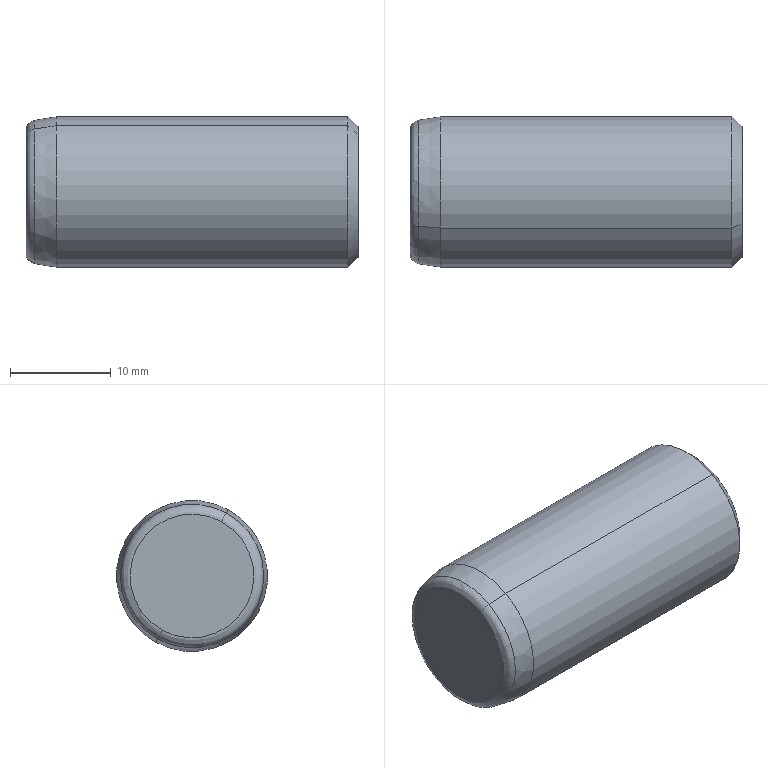Part | STEP file | DOWEL PIN(DOWEL PIN(Φ15×33
)) | 1 solid | 14 faces | box 33 x 15 x 15 mm | volume 5582 mm3 | cone 6 | cylinder 4 | torus 2 | plane 2 | commonest cylinder face diameters 5 x2 15 x2